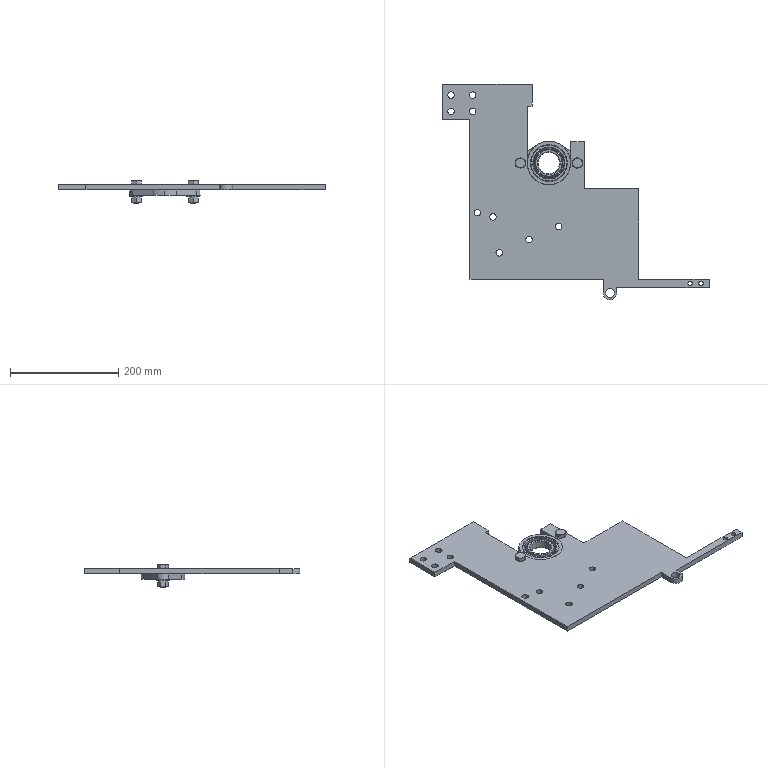Part | SolidWorks | 9 solids | 465 faces | box 490.997 x 397.445 x 42.5 mm | volume 898978 mm3 | cone 136 | plane 107 | sphere 96 | cylinder 78 | torus 48 | commonest cylinder face diameters 12 x34 8 x4 13 x4 18 x4 24 x4 48.8 x4